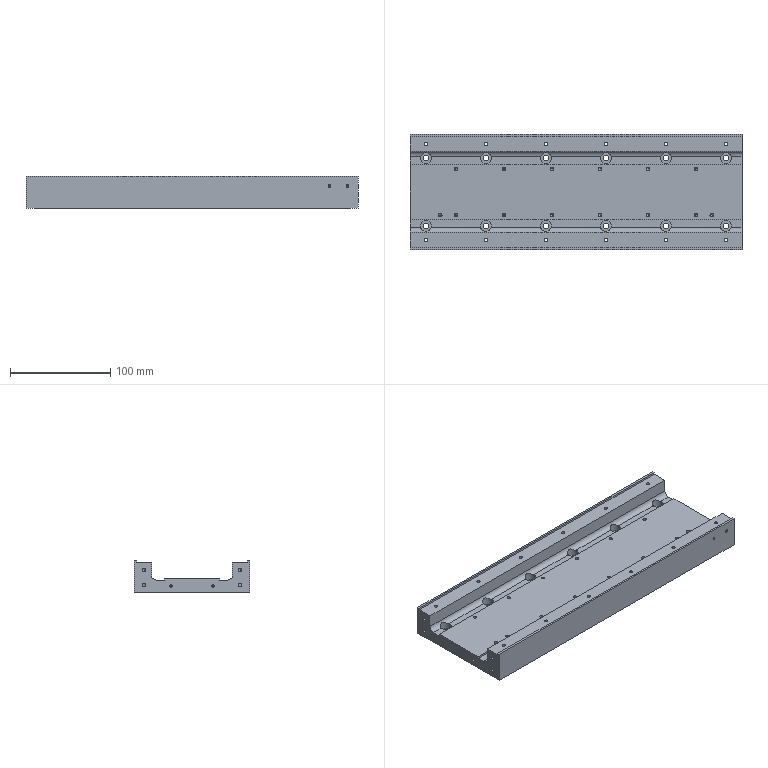Part | STEP file | 1 solid | 335 faces | box 332 x 115 x 32 mm | volume 511026 mm3 | cylinder 192 | plane 91 | cone 52 | commonest cylinder face diameters 3.3 x70 10 x58 5.5 x24 11 x24 2.5 x8 4 x4